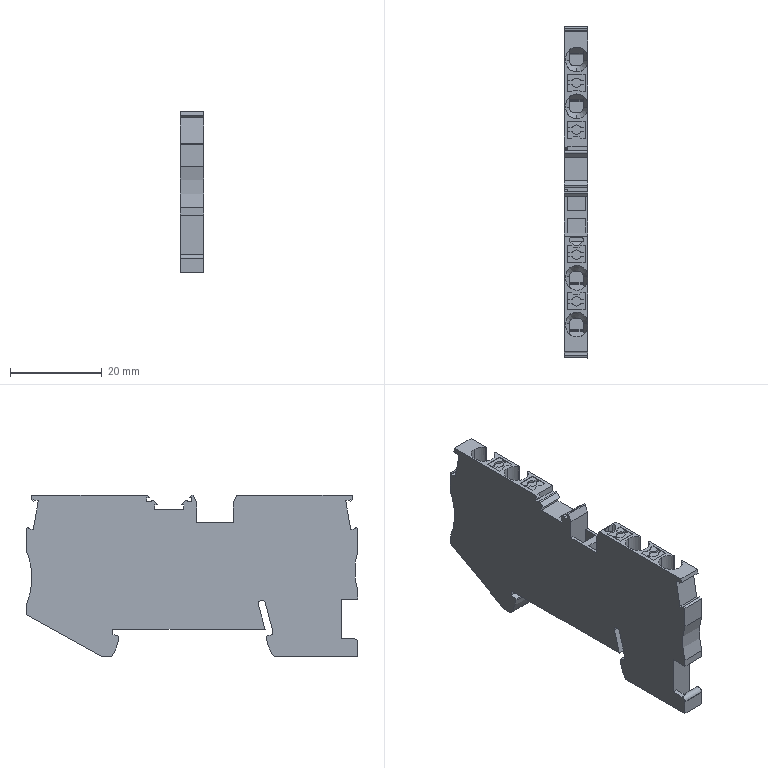Part | STEP file | Straight-through terminal block PT2,5-QUATTRO-3209578 | 1 solid | 262 faces | box 5.15 x 72.2 x 35.25 mm | volume 9561 mm3 | plane 196 | cylinder 47 | spline 13 | cone 6 | commonest cylinder face diameters 2 x20 4.8 x12 1.8 x3 30 x3 0.6 x2 1 x2